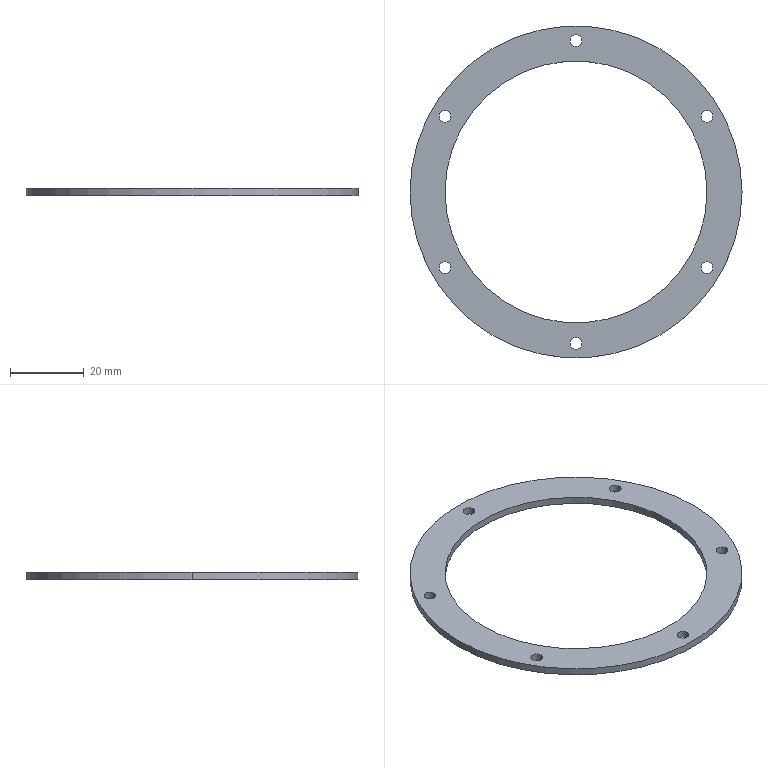Part | SolidWorks | features BaseBody 1 | 1 solid | 18 faces | box 90 x 90 x 2 mm | volume 4709 mm3 | cylinder 16 | plane 2 | commonest cylinder face diameters 3.2 x12 71 x2 90 x2
STEP:
#1=CARTESIAN_POINT('',(-33.907,20.5,2.));
#2=VERTEX_POINT('',#1);
#3=CARTESIAN_POINT('',(-37.107,20.5,2.));
#4=VERTEX_POINT('',#3);
#5=CARTESIAN_POINT('',(-35.507,20.5,2.));
#6=DIRECTION('',(0.,0.,-1.));
#7=DIRECTION('',(-1.,0.,0.));
#8=AXIS2_PLACEMENT_3D('',#5,#6,#7);
#9=CIRCLE('',#8,1.6);
#10=EDGE_CURVE('',#2,#4,#9,.T.);
#11=ORIENTED_EDGE('',*,*,#10,.F.);
#12=CARTESIAN_POINT('',(-33.907,20.5,0.));
#13=VERTEX_POINT('',#12);
#14=CARTESIAN_POINT('',(-33.907,20.5,2.));
#15=DIRECTION('',(0.,0.,-1.));
#16=VECTOR('',#15,1000.);
#17=LINE('',#14,#16);
#18=EDGE_CURVE('',#2,#13,#17,.T.);
#19=ORIENTED_EDGE('',*,*,#18,.T.);
#20=CARTESIAN_POINT('',(-37.107,20.5,0.));
#21=VERTEX_POINT('',#20);
#22=CARTESIAN_POINT('',(-35.507,20.5,0.));
#23=DIRECTION('',(0.,0.,1.));
#24=DIRECTION('',(-1.,0.,0.));
#25=AXIS2_PLACEMENT_3D('',#22,#23,#24);
#26=CIRCLE('',#25,1.6);
#27=EDGE_CURVE('',#21,#13,#26,.T.);
#28=ORIENTED_EDGE('',*,*,#27,.F.);
#29=CARTESIAN_POINT('',(-37.107,20.5,2.));
#30=DIRECTION('',(0.,0.,-1.));
#31=VECTOR('',#30,1000.);
#32=LINE('',#29,#31);
#33=EDGE_CURVE('',#4,#21,#32,.T.);
#34=ORIENTED_EDGE('',*,*,#33,.F.);
#35=EDGE_LOOP('',(#11,#19,#28,#34));
#36=FACE_OUTER_BOUND('',#35,.T.);
#37=CARTESIAN_POINT('',(-35.507,20.5,2.));
#38=DIRECTION('',(0.,0.,-1.));
#39=DIRECTION('',(-1.,0.,0.));
#40=AXIS2_PLACEMENT_3D('',#37,#38,#39);
#41=CYLINDRICAL_SURFACE('',#40,1.6);
#42=ADVANCED_FACE('',(#36),#41,.F.);
#43=CARTESIAN_POINT('',(1.6,-41.,2.));
#44=VERTEX_POINT('',#43);
#45=CARTESIAN_POINT('',(-1.6,-41.,2.));
#46=VERTEX_POINT('',#45);
#47=CARTESIAN_POINT('',(0.,-41.,2.));
#48=DIRECTION('',(0.,0.,-1.));
#49=DIRECTION('',(-1.,0.,0.));
#50=AXIS2_PLACEMENT_3D('',#47,#48,#49);
#51=CIRCLE('',#50,1.6);
#52=EDGE_CURVE('',#44,#46,#51,.T.);
#53=ORIENTED_EDGE('',*,*,#52,.F.);
#54=CARTESIAN_POINT('',(1.6,-41.,0.));
#55=VERTEX_POINT('',#54);
#56=CARTESIAN_POINT('',(1.6,-41.,2.));
#57=DIRECTION('',(0.,0.,-1.));
#58=VECTOR('',#57,1000.);
#59=LINE('',#56,#58);
#60=EDGE_CURVE('',#44,#55,#59,.T.);
#61=ORIENTED_EDGE('',*,*,#60,.T.);
#62=CARTESIAN_POINT('',(-1.6,-41.,0.));
#63=VERTEX_POINT('',#62);
#64=CARTESIAN_POINT('',(0.,-41.,0.));
#65=DIRECTION('',(0.,0.,1.));
#66=DIRECTION('',(-1.,0.,0.));
#67=AXIS2_PLACEMENT_3D('',#64,#65,#66);
#68=CIRCLE('',#67,1.6);
#69=EDGE_CURVE('',#63,#55,#68,.T.);
#70=ORIENTED_EDGE('',*,*,#69,.F.);
#71=CARTESIAN_POINT('',(-1.6,-41.,2.));
#72=DIRECTION('',(0.,0.,-1.));
#73=VECTOR('',#72,1000.);
#74=LINE('',#71,#73);
#75=EDGE_CURVE('',#46,#63,#74,.T.);
#76=ORIENTED_EDGE('',*,*,#75,.F.);
#77=EDGE_LOOP('',(#53,#61,#70,#76));
#78=FACE_OUTER_BOUND('',#77,.T.);
#79=CARTESIAN_POINT('',(0.,-41.,2.));
#80=DIRECTION('',(0.,0.,-1.));
#81=DIRECTION('',(-1.,0.,0.));
#82=AXIS2_PLACEMENT_3D('',#79,#80,#81);
#83=CYLINDRICAL_SURFACE('',#82,1.6);
#84=ADVANCED_FACE('',(#78),#83,.F.);
#85=CARTESIAN_POINT('',(37.107,20.5,2.));
#86=VERTEX_POINT('',#85);
#87=CARTESIAN_POINT('',(33.907,20.5,2.));
#88=VERTEX_POINT('',#87);
#89=CARTESIAN_POINT('',(35.507,20.5,2.));
#90=DIRECTION('',(0.,0.,-1.));
#91=DIRECTION('',(-1.,0.,0.));
#92=AXIS2_PLACEMENT_3D('',#89,#90,#91);
#93=CIRCLE('',#92,1.6);
#94=EDGE_CURVE('',#86,#88,#93,.T.);
#95=ORIENTED_EDGE('',*,*,#94,.F.);
#96=CARTESIAN_POINT('',(37.107,20.5,0.));
#97=VERTEX_POINT('',#96);
#98=CARTESIAN_POINT('',(37.107,20.5,2.));
#99=DIRECTION('',(0.,0.,-1.));
#100=VECTOR('',#99,1000.);
#101=LINE('',#98,#100);
#102=EDGE_CURVE('',#86,#97,#101,.T.);
#103=ORIENTED_EDGE('',*,*,#102,.T.);
#104=CARTESIAN_POINT('',(33.907,20.5,0.));
#105=VERTEX_POINT('',#104);
#106=CARTESIAN_POINT('',(35.507,20.5,0.));
#107=DIRECTION('',(0.,0.,1.));
#108=DIRECTION('',(-1.,0.,0.));
#109=AXIS2_PLACEMENT_3D('',#106,#107,#108);
#110=CIRCLE('',#109,1.6);
#111=EDGE_CURVE('',#105,#97,#110,.T.);
#112=ORIENTED_EDGE('',*,*,#111,.F.);
#113=CARTESIAN_POINT('',(33.907,20.5,2.));
#114=DIRECTION('',(0.,0.,-1.));
#115=VECTOR('',#114,1000.);
#116=LINE('',#113,#115);
#117=EDGE_CURVE('',#88,#105,#116,.T.);
#118=ORIENTED_EDGE('',*,*,#117,.F.);
#119=EDGE_LOOP('',(#95,#103,#112,#118));
#120=FACE_OUTER_BOUND('',#119,.T.);
#121=CARTESIAN_POINT('',(35.507,20.5,2.));
#122=DIRECTION('',(0.,0.,-1.));
#123=DIRECTION('',(-1.,0.,0.));
#124=AXIS2_PLACEMENT_3D('',#121,#122,#123);
#125=CYLINDRICAL_SURFACE('',#124,1.6);
#126=ADVANCED_FACE('',(#120),#125,.F.);
#127=CARTESIAN_POINT('',(35.5,0.,2.));
#128=VERTEX_POINT('',#127);
#129=CARTESIAN_POINT('',(-35.5,0.,2.));
#130=VERTEX_POINT('',#129);
#131=CARTESIAN_POINT('',(0.,0.,2.));
#132=DIRECTION('',(0.,0.,-1.));
#133=DIRECTION('',(-1.,0.,0.));
#134=AXIS2_PLACEMENT_3D('',#131,#132,#133);
#135=CIRCLE('',#134,35.5);
#136=EDGE_CURVE('',#128,#130,#135,.T.);
#137=ORIENTED_EDGE('',*,*,#136,.F.);
#138=CARTESIAN_POINT('',(35.5,0.,0.));
#139=VERTEX_POINT('',#138);
#140=CARTESIAN_POINT('',(35.5,0.,2.));
#141=DIRECTION('',(0.,0.,-1.));
#142=VECTOR('',#141,1000.);
#143=LINE('',#140,#142);
#144=EDGE_CURVE('',#128,#139,#143,.T.);
#145=ORIENTED_EDGE('',*,*,#144,.T.);
#146=CARTESIAN_POINT('',(-35.5,0.,0.));
#147=VERTEX_POINT('',#146);
#148=CARTESIAN_POINT('',(0.,0.,0.));
#149=DIRECTION('',(0.,0.,1.));
#150=DIRECTION('',(-1.,0.,0.));
#151=AXIS2_PLACEMENT_3D('',#148,#149,#150);
#152=CIRCLE('',#151,35.5);
#153=EDGE_CURVE('',#147,#139,#152,.T.);
#154=ORIENTED_EDGE('',*,*,#153,.F.);
#155=CARTESIAN_POINT('',(-35.5,0.,2.));
#156=DIRECTION('',(0.,0.,-1.));
#157=VECTOR('',#156,1000.);
#158=LINE('',#155,#157);
#159=EDGE_CURVE('',#130,#147,#158,.T.);
#160=ORIENTED_EDGE('',*,*,#159,.F.);
#161=EDGE_LOOP('',(#137,#145,#154,#160));
#162=FACE_OUTER_BOUND('',#161,.T.);
#163=CARTESIAN_POINT('',(0.,0.,2.));
#164=DIRECTION('',(0.,0.,-1.));
#165=DIRECTION('',(-1.,0.,0.));
#166=AXIS2_PLACEMENT_3D('',#163,#164,#165);
#167=CYLINDRICAL_SURFACE('',#166,35.5);
#168=ADVANCED_FACE('',(#162),#167,.F.);
#169=CARTESIAN_POINT('',(45.,0.,2.));
#170=VERTEX_POINT('',#169);
#171=CARTESIAN_POINT('',(-45.,0.,2.));
#172=VERTEX_POINT('',#171);
#173=CARTESIAN_POINT('',(0.,0.,2.));
#174=DIRECTION('',(0.,0.,1.));
#175=DIRECTION('',(-1.,0.,0.));
#176=AXIS2_PLACEMENT_3D('',#173,#174,#175);
#177=CIRCLE('',#176,45.);
#178=EDGE_CURVE('',#170,#172,#177,.T.);
#179=ORIENTED_EDGE('',*,*,#178,.F.);
#180=CARTESIAN_POINT('',(45.,0.,0.));
#181=VERTEX_POINT('',#180);
#182=CARTESIAN_POINT('',(45.,0.,2.));
#183=DIRECTION('',(0.,0.,-1.));
#184=VECTOR('',#183,1000.);
#185=LINE('',#182,#184);
#186=EDGE_CURVE('',#170,#181,#185,.T.);
#187=ORIENTED_EDGE('',*,*,#186,.T.);
#188=CARTESIAN_POINT('',(-45.,0.,0.));
#189=VERTEX_POINT('',#188);
#190=CARTESIAN_POINT('',(0.,0.,0.));
#191=DIRECTION('',(0.,0.,1.));
#192=DIRECTION('',(-1.,0.,0.));
#193=AXIS2_PLACEMENT_3D('',#190,#191,#192);
#194=CIRCLE('',#193,45.);
#195=EDGE_CURVE('',#181,#189,#194,.T.);
#196=ORIENTED_EDGE('',*,*,#195,.T.);
#197=CARTESIAN_POINT('',(-45.,0.,2.));
#198=DIRECTION('',(0.,0.,-1.));
#199=VECTOR('',#198,1000.);
#200=LINE('',#197,#199);
#201=EDGE_CURVE('',#172,#189,#200,.T.);
#202=ORIENTED_EDGE('',*,*,#201,.F.);
#203=EDGE_LOOP('',(#179,#187,#196,#202));
#204=FACE_OUTER_BOUND('',#203,.T.);
#205=CARTESIAN_POINT('',(0.,0.,2.));
#206=DIRECTION('',(0.,0.,-1.));
#207=DIRECTION('',(-1.,0.,0.));
#208=AXIS2_PLACEMENT_3D('',#205,#206,#207);
#209=CYLINDRICAL_SURFACE('',#208,45.);
#210=ADVANCED_FACE('',(#204),#209,.T.);
#211=CARTESIAN_POINT('',(1.6,41.,2.));
#212=VERTEX_POINT('',#211);
#213=CARTESIAN_POINT('',(-1.6,41.,2.));
#214=VERTEX_POINT('',#213);
#215=CARTESIAN_POINT('',(0.,41.,2.));
#216=DIRECTION('',(0.,0.,-1.));
#217=DIRECTION('',(-1.,0.,0.));
#218=AXIS2_PLACEMENT_3D('',#215,#216,#217);
#219=CIRCLE('',#218,1.6);
#220=EDGE_CURVE('',#212,#214,#219,.T.);
#221=ORIENTED_EDGE('',*,*,#220,.F.);
#222=CARTESIAN_POINT('',(1.6,41.,0.));
#223=VERTEX_POINT('',#222);
#224=CARTESIAN_POINT('',(1.6,41.,2.));
#225=DIRECTION('',(0.,0.,-1.));
#226=VECTOR('',#225,1000.);
#227=LINE('',#224,#226);
#228=EDGE_CURVE('',#212,#223,#227,.T.);
#229=ORIENTED_EDGE('',*,*,#228,.T.);
#230=CARTESIAN_POINT('',(-1.6,41.,0.));
#231=VERTEX_POINT('',#230);
#232=CARTESIAN_POINT('',(0.,41.,0.));
#233=DIRECTION('',(0.,0.,1.));
#234=DIRECTION('',(-1.,0.,0.));
#235=AXIS2_PLACEMENT_3D('',#232,#233,#234);
#236=CIRCLE('',#235,1.6);
#237=EDGE_CURVE('',#231,#223,#236,.T.);
#238=ORIENTED_EDGE('',*,*,#237,.F.);
#239=CARTESIAN_POINT('',(-1.6,41.,2.));
#240=DIRECTION('',(0.,0.,-1.));
#241=VECTOR('',#240,1000.);
#242=LINE('',#239,#241);
#243=EDGE_CURVE('',#214,#231,#242,.T.);
#244=ORIENTED_EDGE('',*,*,#243,.F.);
#245=EDGE_LOOP('',(#221,#229,#238,#244));
#246=FACE_OUTER_BOUND('',#245,.T.);
#247=CARTESIAN_POINT('',(0.,41.,2.));
#248=DIRECTION('',(0.,0.,-1.));
#249=DIRECTION('',(-1.,0.,0.));
#250=AXIS2_PLACEMENT_3D('',#247,#248,#249);
#251=CYLINDRICAL_SURFACE('',#250,1.6);
#252=ADVANCED_FACE('',(#246),#251,.F.);
#253=CARTESIAN_POINT('',(37.107,-20.5,2.));
#254=VERTEX_POINT('',#253);
#255=CARTESIAN_POINT('',(33.907,-20.5,2.));
#256=VERTEX_POINT('',#255);
#257=CARTESIAN_POINT('',(35.507,-20.5,2.));
#258=DIRECTION('',(0.,0.,-1.));
#259=DIRECTION('',(-1.,0.,0.));
#260=AXIS2_PLACEMENT_3D('',#257,#258,#259);
#261=CIRCLE('',#260,1.6);
#262=EDGE_CURVE('',#254,#256,#261,.T.);
#263=ORIENTED_EDGE('',*,*,#262,.F.);
#264=CARTESIAN_POINT('',(37.107,-20.5,0.));
#265=VERTEX_POINT('',#264);
#266=CARTESIAN_POINT('',(37.107,-20.5,2.));
#267=DIRECTION('',(0.,0.,-1.));
#268=VECTOR('',#267,1000.);
#269=LINE('',#266,#268);
#270=EDGE_CURVE('',#254,#265,#269,.T.);
#271=ORIENTED_EDGE('',*,*,#270,.T.);
#272=CARTESIAN_POINT('',(33.907,-20.5,0.));
#273=VERTEX_POINT('',#272);
#274=CARTESIAN_POINT('',(35.507,-20.5,0.));
#275=DIRECTION('',(0.,0.,1.));
#276=DIRECTION('',(-1.,0.,0.));
#277=AXIS2_PLACEMENT_3D('',#274,#275,#276);
#278=CIRCLE('',#277,1.6);
#279=EDGE_CURVE('',#273,#265,#278,.T.);
#280=ORIENTED_EDGE('',*,*,#279,.F.);
#281=CARTESIAN_POINT('',(33.907,-20.5,2.));
#282=DIRECTION('',(0.,0.,-1.));
#283=VECTOR('',#282,1000.);
#284=LINE('',#281,#283);
#285=EDGE_CURVE('',#256,#273,#284,.T.);
#286=ORIENTED_EDGE('',*,*,#285,.F.);
#287=EDGE_LOOP('',(#263,#271,#280,#286));
#288=FACE_OUTER_BOUND('',#287,.T.);
#289=CARTESIAN_POINT('',(35.507,-20.5,2.));
#290=DIRECTION('',(0.,0.,-1.));
#291=DIRECTION('',(-1.,0.,0.));
#292=AXIS2_PLACEMENT_3D('',#289,#290,#291);
#293=CYLINDRICAL_SURFACE('',#292,1.6);
#294=ADVANCED_FACE('',(#288),#293,.F.);
#295=CARTESIAN_POINT('',(-33.907,-20.5,2.));
#296=VERTEX_POINT('',#295);
#297=CARTESIAN_POINT('',(-37.107,-20.5,2.));
#298=VERTEX_POINT('',#297);
#299=CARTESIAN_POINT('',(-35.507,-20.5,2.));
#300=DIRECTION('',(0.,0.,-1.));
#301=DIRECTION('',(-1.,0.,0.));
#302=AXIS2_PLACEMENT_3D('',#299,#300,#301);
#303=CIRCLE('',#302,1.6);
#304=EDGE_CURVE('',#296,#298,#303,.T.);
#305=ORIENTED_EDGE('',*,*,#304,.F.);
#306=CARTESIAN_POINT('',(-33.907,-20.5,0.));
#307=VERTEX_POINT('',#306);
#308=CARTESIAN_POINT('',(-33.907,-20.5,2.));
#309=DIRECTION('',(0.,0.,-1.));
#310=VECTOR('',#309,1000.);
#311=LINE('',#308,#310);
#312=EDGE_CURVE('',#296,#307,#311,.T.);
#313=ORIENTED_EDGE('',*,*,#312,.T.);
#314=CARTESIAN_POINT('',(-37.107,-20.5,0.));
#315=VERTEX_POINT('',#314);
#316=CARTESIAN_POINT('',(-35.507,-20.5,0.));
#317=DIRECTION('',(0.,0.,1.));
#318=DIRECTION('',(-1.,0.,0.));
#319=AXIS2_PLACEMENT_3D('',#316,#317,#318);
#320=CIRCLE('',#319,1.6);
#321=EDGE_CURVE('',#315,#307,#320,.T.);
#322=ORIENTED_EDGE('',*,*,#321,.F.);
#323=CARTESIAN_POINT('',(-37.107,-20.5,2.));
#324=DIRECTION('',(0.,0.,-1.));
#325=VECTOR('',#324,1000.);
#326=LINE('',#323,#325);
#327=EDGE_CURVE('',#298,#315,#326,.T.);
#328=ORIENTED_EDGE('',*,*,#327,.F.);
#329=EDGE_LOOP('',(#305,#313,#322,#328));
#330=FACE_OUTER_BOUND('',#329,.T.);
#331=CARTESIAN_POINT('',(-35.507,-20.5,2.));
#332=DIRECTION('',(0.,0.,-1.));
#333=DIRECTION('',(-1.,0.,0.));
#334=AXIS2_PLACEMENT_3D('',#331,#332,#333);
#335=CYLINDRICAL_SURFACE('',#334,1.6);
#336=ADVANCED_FACE('',(#330),#335,.F.);
#337=CARTESIAN_POINT('',(-35.507,20.5,2.));
#338=DIRECTION('',(0.,0.,-1.));
#339=DIRECTION('',(-1.,0.,0.));
#340=AXIS2_PLACEMENT_3D('',#337,#338,#339);
#341=CIRCLE('',#340,1.6);
#342=EDGE_CURVE('',#4,#2,#341,.T.);
#343=ORIENTED_EDGE('',*,*,#342,.T.);
#344=ORIENTED_EDGE('',*,*,#10,.T.);
#345=EDGE_LOOP('',(#343,#344));
#346=FACE_BOUND('',#345,.T.);
#347=CARTESIAN_POINT('',(0.,-41.,2.));
#348=DIRECTION('',(0.,0.,-1.));
#349=DIRECTION('',(-1.,0.,0.));
#350=AXIS2_PLACEMENT_3D('',#347,#348,#349);
#351=CIRCLE('',#350,1.6);
#352=EDGE_CURVE('',#46,#44,#351,.T.);
#353=ORIENTED_EDGE('',*,*,#352,.T.);
#354=ORIENTED_EDGE('',*,*,#52,.T.);
#355=EDGE_LOOP('',(#353,#354));
#356=FACE_BOUND('',#355,.T.);
#357=CARTESIAN_POINT('',(35.507,20.5,2.));
#358=DIRECTION('',(0.,0.,-1.));
#359=DIRECTION('',(-1.,0.,0.));
#360=AXIS2_PLACEMENT_3D('',#357,#358,#359);
#361=CIRCLE('',#360,1.6);
#362=EDGE_CURVE('',#88,#86,#361,.T.);
#363=ORIENTED_EDGE('',*,*,#362,.T.);
#364=ORIENTED_EDGE('',*,*,#94,.T.);
#365=EDGE_LOOP('',(#363,#364));
#366=FACE_BOUND('',#365,.T.);
#367=CARTESIAN_POINT('',(0.,0.,2.));
#368=DIRECTION('',(0.,0.,-1.));
#369=DIRECTION('',(-1.,0.,0.));
#370=AXIS2_PLACEMENT_3D('',#367,#368,#369);
#371=CIRCLE('',#370,35.5);
#372=EDGE_CURVE('',#130,#128,#371,.T.);
#373=ORIENTED_EDGE('',*,*,#372,.T.);
#374=ORIENTED_EDGE('',*,*,#136,.T.);
#375=EDGE_LOOP('',(#373,#374));
#376=FACE_BOUND('',#375,.T.);
#377=CARTESIAN_POINT('',(0.,0.,2.));
#378=DIRECTION('',(0.,0.,1.));
#379=DIRECTION('',(-1.,0.,0.));
#380=AXIS2_PLACEMENT_3D('',#377,#378,#379);
#381=CIRCLE('',#380,45.);
#382=EDGE_CURVE('',#172,#170,#381,.T.);
#383=ORIENTED_EDGE('',*,*,#382,.T.);
#384=ORIENTED_EDGE('',*,*,#178,.T.);
#385=EDGE_LOOP('',(#383,#384));
#386=FACE_OUTER_BOUND('',#385,.T.);
#387=CARTESIAN_POINT('',(0.,41.,2.));
#388=DIRECTION('',(0.,0.,-1.));
#389=DIRECTION('',(-1.,0.,0.));
#390=AXIS2_PLACEMENT_3D('',#387,#388,#389);
#391=CIRCLE('',#390,1.6);
#392=EDGE_CURVE('',#214,#212,#391,.T.);
#393=ORIENTED_EDGE('',*,*,#392,.T.);
#394=ORIENTED_EDGE('',*,*,#220,.T.);
#395=EDGE_LOOP('',(#393,#394));
#396=FACE_BOUND('',#395,.T.);
#397=CARTESIAN_POINT('',(35.507,-20.5,2.));
#398=DIRECTION('',(0.,0.,-1.));
#399=DIRECTION('',(-1.,0.,0.));
#400=AXIS2_PLACEMENT_3D('',#397,#398,#399);
#401=CIRCLE('',#400,1.6);
#402=EDGE_CURVE('',#256,#254,#401,.T.);
#403=ORIENTED_EDGE('',*,*,#402,.T.);
#404=ORIENTED_EDGE('',*,*,#262,.T.);
#405=EDGE_LOOP('',(#403,#404));
#406=FACE_BOUND('',#405,.T.);
#407=CARTESIAN_POINT('',(-35.507,-20.5,2.));
#408=DIRECTION('',(0.,0.,-1.));
#409=DIRECTION('',(-1.,0.,0.));
#410=AXIS2_PLACEMENT_3D('',#407,#408,#409);
#411=CIRCLE('',#410,1.6);
#412=EDGE_CURVE('',#298,#296,#411,.T.);
#413=ORIENTED_EDGE('',*,*,#412,.T.);
#414=ORIENTED_EDGE('',*,*,#304,.T.);
#415=EDGE_LOOP('',(#413,#414));
#416=FACE_BOUND('',#415,.T.);
#417=CARTESIAN_POINT('',(0.,0.,2.));
#418=DIRECTION('',(0.,0.,1.));
#419=DIRECTION('',(1.,0.,0.));
#420=AXIS2_PLACEMENT_3D('',#417,#418,#419);
#421=PLANE('',#420);
#422=ADVANCED_FACE('',(#346,#356,#366,#376,#386,#396,#406,#416),#421,.T.);
#423=ORIENTED_EDGE('',*,*,#18,.F.);
#424=ORIENTED_EDGE('',*,*,#342,.F.);
#425=ORIENTED_EDGE('',*,*,#33,.T.);
#426=CARTESIAN_POINT('',(-35.507,20.5,0.));
#427=DIRECTION('',(0.,0.,1.));
#428=DIRECTION('',(-1.,0.,0.));
#429=AXIS2_PLACEMENT_3D('',#426,#427,#428);
#430=CIRCLE('',#429,1.6);
#431=EDGE_CURVE('',#13,#21,#430,.T.);
#432=ORIENTED_EDGE('',*,*,#431,.F.);
#433=EDGE_LOOP('',(#423,#424,#425,#432));
#434=FACE_OUTER_BOUND('',#433,.T.);
#435=CARTESIAN_POINT('',(-35.507,20.5,2.));
#436=DIRECTION('',(0.,0.,-1.));
#437=DIRECTION('',(-1.,0.,0.));
#438=AXIS2_PLACEMENT_3D('',#435,#436,#437);
#439=CYLINDRICAL_SURFACE('',#438,1.6);
#440=ADVANCED_FACE('',(#434),#439,.F.);
#441=ORIENTED_EDGE('',*,*,#60,.F.);
#442=ORIENTED_EDGE('',*,*,#352,.F.);
#443=ORIENTED_EDGE('',*,*,#75,.T.);
#444=CARTESIAN_POINT('',(0.,-41.,0.));
#445=DIRECTION('',(0.,0.,1.));
#446=DIRECTION('',(-1.,0.,0.));
#447=AXIS2_PLACEMENT_3D('',#444,#445,#446);
#448=CIRCLE('',#447,1.6);
#449=EDGE_CURVE('',#55,#63,#448,.T.);
#450=ORIENTED_EDGE('',*,*,#449,.F.);
#451=EDGE_LOOP('',(#441,#442,#443,#450));
#452=FACE_OUTER_BOUND('',#451,.T.);
#453=CARTESIAN_POINT('',(0.,-41.,2.));
#454=DIRECTION('',(0.,0.,-1.));
#455=DIRECTION('',(-1.,0.,0.));
#456=AXIS2_PLACEMENT_3D('',#453,#454,#455);
#457=CYLINDRICAL_SURFACE('',#456,1.6);
#458=ADVANCED_FACE('',(#452),#457,.F.);
#459=ORIENTED_EDGE('',*,*,#102,.F.);
#460=ORIENTED_EDGE('',*,*,#362,.F.);
#461=ORIENTED_EDGE('',*,*,#117,.T.);
#462=CARTESIAN_POINT('',(35.507,20.5,0.));
#463=DIRECTION('',(0.,0.,1.));
#464=DIRECTION('',(-1.,0.,0.));
#465=AXIS2_PLACEMENT_3D('',#462,#463,#464);
#466=CIRCLE('',#465,1.6);
#467=EDGE_CURVE('',#97,#105,#466,.T.);
#468=ORIENTED_EDGE('',*,*,#467,.F.);
#469=EDGE_LOOP('',(#459,#460,#461,#468));
#470=FACE_OUTER_BOUND('',#469,.T.);
#471=CARTESIAN_POINT('',(35.507,20.5,2.));
#472=DIRECTION('',(0.,0.,-1.));
#473=DIRECTION('',(-1.,0.,0.));
#474=AXIS2_PLACEMENT_3D('',#471,#472,#473);
#475=CYLINDRICAL_SURFACE('',#474,1.6);
#476=ADVANCED_FACE('',(#470),#475,.F.);
#477=ORIENTED_EDGE('',*,*,#144,.F.);
#478=ORIENTED_EDGE('',*,*,#372,.F.);
#479=ORIENTED_EDGE('',*,*,#159,.T.);
#480=CARTESIAN_POINT('',(0.,0.,0.));
#481=DIRECTION('',(0.,0.,1.));
#482=DIRECTION('',(-1.,0.,0.));
#483=AXIS2_PLACEMENT_3D('',#480,#481,#482);
#484=CIRCLE('',#483,35.5);
#485=EDGE_CURVE('',#139,#147,#484,.T.);
#486=ORIENTED_EDGE('',*,*,#485,.F.);
#487=EDGE_LOOP('',(#477,#478,#479,#486));
#488=FACE_OUTER_BOUND('',#487,.T.);
#489=CARTESIAN_POINT('',(0.,0.,2.));
#490=DIRECTION('',(0.,0.,-1.));
#491=DIRECTION('',(-1.,0.,0.));
#492=AXIS2_PLACEMENT_3D('',#489,#490,#491);
#493=CYLINDRICAL_SURFACE('',#492,35.5);
#494=ADVANCED_FACE('',(#488),#493,.F.);
#495=ORIENTED_EDGE('',*,*,#186,.F.);
#496=ORIENTED_EDGE('',*,*,#382,.F.);
#497=ORIENTED_EDGE('',*,*,#201,.T.);
#498=CARTESIAN_POINT('',(0.,0.,0.));
#499=DIRECTION('',(0.,0.,1.));
#500=DIRECTION('',(-1.,0.,0.));
#501=AXIS2_PLACEMENT_3D('',#498,#499,#500);
#502=CIRCLE('',#501,45.);
#503=EDGE_CURVE('',#189,#181,#502,.T.);
#504=ORIENTED_EDGE('',*,*,#503,.T.);
#505=EDGE_LOOP('',(#495,#496,#497,#504));
#506=FACE_OUTER_BOUND('',#505,.T.);
#507=CARTESIAN_POINT('',(0.,0.,2.));
#508=DIRECTION('',(0.,0.,-1.));
#509=DIRECTION('',(-1.,0.,0.));
#510=AXIS2_PLACEMENT_3D('',#507,#508,#509);
#511=CYLINDRICAL_SURFACE('',#510,45.);
#512=ADVANCED_FACE('',(#506),#511,.T.);
#513=ORIENTED_EDGE('',*,*,#228,.F.);
#514=ORIENTED_EDGE('',*,*,#392,.F.);
#515=ORIENTED_EDGE('',*,*,#243,.T.);
#516=CARTESIAN_POINT('',(0.,41.,0.));
#517=DIRECTION('',(0.,0.,1.));
#518=DIRECTION('',(-1.,0.,0.));
#519=AXIS2_PLACEMENT_3D('',#516,#517,#518);
#520=CIRCLE('',#519,1.6);
#521=EDGE_CURVE('',#223,#231,#520,.T.);
#522=ORIENTED_EDGE('',*,*,#521,.F.);
#523=EDGE_LOOP('',(#513,#514,#515,#522));
#524=FACE_OUTER_BOUND('',#523,.T.);
#525=CARTESIAN_POINT('',(0.,41.,2.));
#526=DIRECTION('',(0.,0.,-1.));
#527=DIRECTION('',(-1.,0.,0.));
#528=AXIS2_PLACEMENT_3D('',#525,#526,#527);
#529=CYLINDRICAL_SURFACE('',#528,1.6);
#530=ADVANCED_FACE('',(#524),#529,.F.);
#531=ORIENTED_EDGE('',*,*,#270,.F.);
#532=ORIENTED_EDGE('',*,*,#402,.F.);
#533=ORIENTED_EDGE('',*,*,#285,.T.);
#534=CARTESIAN_POINT('',(35.507,-20.5,0.));
#535=DIRECTION('',(0.,0.,1.));
#536=DIRECTION('',(-1.,0.,0.));
#537=AXIS2_PLACEMENT_3D('',#534,#535,#536);
#538=CIRCLE('',#537,1.6);
#539=EDGE_CURVE('',#265,#273,#538,.T.);
#540=ORIENTED_EDGE('',*,*,#539,.F.);
#541=EDGE_LOOP('',(#531,#532,#533,#540));
#542=FACE_OUTER_BOUND('',#541,.T.);
#543=CARTESIAN_POINT('',(35.507,-20.5,2.));
#544=DIRECTION('',(0.,0.,-1.));
#545=DIRECTION('',(-1.,0.,0.));
#546=AXIS2_PLACEMENT_3D('',#543,#544,#545);
#547=CYLINDRICAL_SURFACE('',#546,1.6);
#548=ADVANCED_FACE('',(#542),#547,.F.);
#549=ORIENTED_EDGE('',*,*,#312,.F.);
#550=ORIENTED_EDGE('',*,*,#412,.F.);
#551=ORIENTED_EDGE('',*,*,#327,.T.);
#552=CARTESIAN_POINT('',(-35.507,-20.5,0.));
#553=DIRECTION('',(0.,0.,1.));
#554=DIRECTION('',(-1.,0.,0.));
#555=AXIS2_PLACEMENT_3D('',#552,#553,#554);
#556=CIRCLE('',#555,1.6);
#557=EDGE_CURVE('',#307,#315,#556,.T.);
#558=ORIENTED_EDGE('',*,*,#557,.F.);
#559=EDGE_LOOP('',(#549,#550,#551,#558));
#560=FACE_OUTER_BOUND('',#559,.T.);
#561=CARTESIAN_POINT('',(-35.507,-20.5,2.));
#562=DIRECTION('',(0.,0.,-1.));
#563=DIRECTION('',(-1.,0.,0.));
#564=AXIS2_PLACEMENT_3D('',#561,#562,#563);
#565=CYLINDRICAL_SURFACE('',#564,1.6);
#566=ADVANCED_FACE('',(#560),#565,.F.);
#567=ORIENTED_EDGE('',*,*,#27,.T.);
#568=ORIENTED_EDGE('',*,*,#431,.T.);
#569=EDGE_LOOP('',(#567,#568));
#570=FACE_BOUND('',#569,.T.);
#571=ORIENTED_EDGE('',*,*,#321,.T.);
#572=ORIENTED_EDGE('',*,*,#557,.T.);
#573=EDGE_LOOP('',(#571,#572));
#574=FACE_BOUND('',#573,.T.);
#575=ORIENTED_EDGE('',*,*,#69,.T.);
#576=ORIENTED_EDGE('',*,*,#449,.T.);
#577=EDGE_LOOP('',(#575,#576));
#578=FACE_BOUND('',#577,.T.);
#579=ORIENTED_EDGE('',*,*,#279,.T.);
#580=ORIENTED_EDGE('',*,*,#539,.T.);
#581=EDGE_LOOP('',(#579,#580));
#582=FACE_BOUND('',#581,.T.);
#583=ORIENTED_EDGE('',*,*,#111,.T.);
#584=ORIENTED_EDGE('',*,*,#467,.T.);
#585=EDGE_LOOP('',(#583,#584));
#586=FACE_BOUND('',#585,.T.);
#587=ORIENTED_EDGE('',*,*,#237,.T.);
#588=ORIENTED_EDGE('',*,*,#521,.T.);
#589=EDGE_LOOP('',(#587,#588));
#590=FACE_BOUND('',#589,.T.);
#591=ORIENTED_EDGE('',*,*,#153,.T.);
#592=ORIENTED_EDGE('',*,*,#485,.T.);
#593=EDGE_LOOP('',(#591,#592));
#594=FACE_BOUND('',#593,.T.);
#595=ORIENTED_EDGE('',*,*,#503,.F.);
#596=ORIENTED_EDGE('',*,*,#195,.F.);
#597=EDGE_LOOP('',(#595,#596));
#598=FACE_OUTER_BOUND('',#597,.T.);
#599=CARTESIAN_POINT('',(0.,0.,0.));
#600=DIRECTION('',(0.,0.,1.));
#601=DIRECTION('',(1.,0.,0.));
#602=AXIS2_PLACEMENT_3D('',#599,#600,#601);
#603=PLANE('',#602);
#604=ADVANCED_FACE('',(#570,#574,#578,#582,#586,#590,#594,#598),#603,.F.);
#605=CLOSED_SHELL('',(#42,#84,#126,#168,#210,#252,#294,#336,#422,#440,#458,#476,#494,#512,#530,#548,#566,#604));
#606=MANIFOLD_SOLID_BREP('',#605);
#607=CARTESIAN_POINT('',(0.,0.,0.));
#608=DIRECTION('',(0.,0.,1.));
#609=DIRECTION('',(1.,0.,0.));
#610=AXIS2_PLACEMENT_3D('',#607,#608,#609);
#611=(LENGTH_UNIT()NAMED_UNIT(*)SI_UNIT(.MILLI.,.METRE.));
#612=UNCERTAINTY_MEASURE_WITH_UNIT(LENGTH_MEASURE(0.00001),#611,'','');
#613=(NAMED_UNIT(*)PLANE_ANGLE_UNIT()SI_UNIT($,.RADIAN.));
#614=(NAMED_UNIT(*)SI_UNIT($,.STERADIAN.)SOLID_ANGLE_UNIT());
#615=(GEOMETRIC_REPRESENTATION_CONTEXT(3)GLOBAL_UNCERTAINTY_ASSIGNED_CONTEXT((#612))GLOBAL_UNIT_ASSIGNED_CONTEXT((#611,#613,#614))REPRESENTATION_CONTEXT('',''));
#616=ADVANCED_BREP_SHAPE_REPRESENTATION('',(#606,#610),#615);